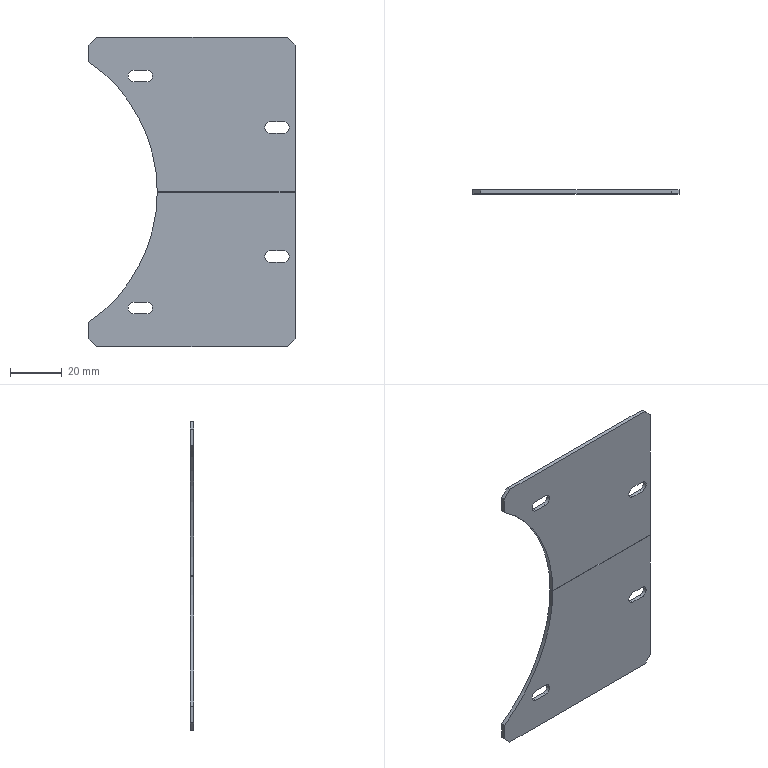Part | SolidWorks | features ICE 6, Chamfer 4, Extrusion 1 | 2 solids | 34 faces | box 80 x 1.5 x 120 mm | volume 11312 mm3 | plane 24 | cylinder 10 | commonest cylinder face diameters 4.5 x8 123 x2
STEP:
#1=CARTESIAN_POINT('',(-249.5,1.5,0.05));
#2=VERTEX_POINT('',#1);
#3=CARTESIAN_POINT('',(-196.,1.5,0.05));
#4=VERTEX_POINT('',#3);
#5=CARTESIAN_POINT('',(-276.,1.5,0.05));
#6=DIRECTION('',(1.,0.,0.));
#7=VECTOR('',#6,1000.);
#8=LINE('',#5,#7);
#9=EDGE_CURVE('',#2,#4,#8,.T.);
#10=ORIENTED_EDGE('',*,*,#9,.T.);
#11=CARTESIAN_POINT('',(-196.,0.,0.05));
#12=VERTEX_POINT('',#11);
#13=CARTESIAN_POINT('',(-196.,0.,0.05));
#14=DIRECTION('',(0.,-1.,0.));
#15=VECTOR('',#14,1000.);
#16=LINE('',#13,#15);
#17=EDGE_CURVE('',#4,#12,#16,.T.);
#18=ORIENTED_EDGE('',*,*,#17,.T.);
#19=CARTESIAN_POINT('',(-249.5,0.,0.05));
#20=VERTEX_POINT('',#19);
#21=CARTESIAN_POINT('',(-276.,0.,0.05));
#22=DIRECTION('',(1.,0.,0.));
#23=VECTOR('',#22,1000.);
#24=LINE('',#21,#23);
#25=EDGE_CURVE('',#20,#12,#24,.T.);
#26=ORIENTED_EDGE('',*,*,#25,.F.);
#27=CARTESIAN_POINT('',(-249.5,-8.5,0.05));
#28=DIRECTION('',(0.,1.,0.));
#29=VECTOR('',#28,1000.);
#30=LINE('',#27,#29);
#31=EDGE_CURVE('',#20,#2,#30,.T.);
#32=ORIENTED_EDGE('',*,*,#31,.T.);
#33=EDGE_LOOP('',(#10,#18,#26,#32));
#34=FACE_OUTER_BOUND('',#33,.T.);
#35=CARTESIAN_POINT('',(-276.,0.,0.05));
#36=DIRECTION('',(0.,0.,1.));
#37=DIRECTION('',(1.,0.,0.));
#38=AXIS2_PLACEMENT_3D('',#35,#36,#37);
#39=PLANE('',#38);
#40=ADVANCED_FACE('',(#34),#39,.F.);
#41=CARTESIAN_POINT('',(-276.,1.5,50.569));
#42=VERTEX_POINT('',#41);
#43=CARTESIAN_POINT('',(-276.,1.5,57.));
#44=VERTEX_POINT('',#43);
#45=CARTESIAN_POINT('',(-276.,1.5,-60.));
#46=DIRECTION('',(0.,0.,1.));
#47=VECTOR('',#46,1000.);
#48=LINE('',#45,#47);
#49=EDGE_CURVE('',#42,#44,#48,.T.);
#50=ORIENTED_EDGE('',*,*,#49,.F.);
#51=CARTESIAN_POINT('',(-276.,0.,50.569));
#52=VERTEX_POINT('',#51);
#53=CARTESIAN_POINT('',(-276.,-8.5,50.569));
#54=DIRECTION('',(0.,-1.,0.));
#55=VECTOR('',#54,1000.);
#56=LINE('',#53,#55);
#57=EDGE_CURVE('',#42,#52,#56,.T.);
#58=ORIENTED_EDGE('',*,*,#57,.T.);
#59=CARTESIAN_POINT('',(-276.,0.,57.));
#60=VERTEX_POINT('',#59);
#61=CARTESIAN_POINT('',(-276.,0.,-60.));
#62=DIRECTION('',(0.,0.,1.));
#63=VECTOR('',#62,1000.);
#64=LINE('',#61,#63);
#65=EDGE_CURVE('',#52,#60,#64,.T.);
#66=ORIENTED_EDGE('',*,*,#65,.T.);
#67=CARTESIAN_POINT('',(-276.,1.5,57.));
#68=DIRECTION('',(0.,1.,0.));
#69=VECTOR('',#68,1000.);
#70=LINE('',#67,#69);
#71=EDGE_CURVE('',#60,#44,#70,.T.);
#72=ORIENTED_EDGE('',*,*,#71,.T.);
#73=EDGE_LOOP('',(#50,#58,#66,#72));
#74=FACE_OUTER_BOUND('',#73,.T.);
#75=CARTESIAN_POINT('',(-276.,1.5,-60.));
#76=DIRECTION('',(1.,0.,0.));
#77=DIRECTION('',(0.,0.,-1.));
#78=AXIS2_PLACEMENT_3D('',#75,#76,#77);
#79=PLANE('',#78);
#80=ADVANCED_FACE('',(#74),#79,.F.);
#81=CARTESIAN_POINT('',(-200.5,1.5,27.25));
#82=VERTEX_POINT('',#81);
#83=CARTESIAN_POINT('',(-200.5,1.5,22.75));
#84=VERTEX_POINT('',#83);
#85=CARTESIAN_POINT('',(-200.5,1.5,25.));
#86=DIRECTION('',(0.,1.,0.));
#87=DIRECTION('',(0.,0.,1.));
#88=AXIS2_PLACEMENT_3D('',#85,#86,#87);
#89=CIRCLE('',#88,2.25);
#90=EDGE_CURVE('',#82,#84,#89,.T.);
#91=ORIENTED_EDGE('',*,*,#90,.F.);
#92=CARTESIAN_POINT('',(-205.5,1.5,27.25));
#93=VERTEX_POINT('',#92);
#94=CARTESIAN_POINT('',(0.,1.5,27.25));
#95=DIRECTION('',(1.,0.,0.));
#96=VECTOR('',#95,1000.);
#97=LINE('',#94,#96);
#98=EDGE_CURVE('',#93,#82,#97,.T.);
#99=ORIENTED_EDGE('',*,*,#98,.F.);
#100=CARTESIAN_POINT('',(-205.5,1.5,22.75));
#101=VERTEX_POINT('',#100);
#102=CARTESIAN_POINT('',(-205.5,1.5,25.));
#103=DIRECTION('',(0.,1.,0.));
#104=DIRECTION('',(0.,0.,1.));
#105=AXIS2_PLACEMENT_3D('',#102,#103,#104);
#106=CIRCLE('',#105,2.25);
#107=EDGE_CURVE('',#101,#93,#106,.T.);
#108=ORIENTED_EDGE('',*,*,#107,.F.);
#109=CARTESIAN_POINT('',(0.,1.5,22.75));
#110=DIRECTION('',(-1.,0.,0.));
#111=VECTOR('',#110,1000.);
#112=LINE('',#109,#111);
#113=EDGE_CURVE('',#84,#101,#112,.T.);
#114=ORIENTED_EDGE('',*,*,#113,.F.);
#115=EDGE_LOOP('',(#91,#99,#108,#114));
#116=FACE_BOUND('',#115,.T.);
#117=CARTESIAN_POINT('',(-273.,1.5,60.));
#118=VERTEX_POINT('',#117);
#119=CARTESIAN_POINT('',(-199.,1.5,60.));
#120=VERTEX_POINT('',#119);
#121=CARTESIAN_POINT('',(-276.,1.5,60.));
#122=DIRECTION('',(1.,0.,0.));
#123=VECTOR('',#122,1000.);
#124=LINE('',#121,#123);
#125=EDGE_CURVE('',#118,#120,#124,.T.);
#126=ORIENTED_EDGE('',*,*,#125,.T.);
#127=CARTESIAN_POINT('',(-196.,1.5,57.));
#128=VERTEX_POINT('',#127);
#129=CARTESIAN_POINT('',(-69.5,1.5,-69.5));
#130=DIRECTION('',(0.7071,0.,-0.7071));
#131=VECTOR('',#130,1000.);
#132=LINE('',#129,#131);
#133=EDGE_CURVE('',#120,#128,#132,.T.);
#134=ORIENTED_EDGE('',*,*,#133,.T.);
#135=CARTESIAN_POINT('',(-196.,1.5,0.));
#136=DIRECTION('',(0.,0.,1.));
#137=VECTOR('',#136,1000.);
#138=LINE('',#135,#137);
#139=EDGE_CURVE('',#4,#128,#138,.T.);
#140=ORIENTED_EDGE('',*,*,#139,.F.);
#141=ORIENTED_EDGE('',*,*,#9,.F.);
#142=CARTESIAN_POINT('',(-311.,1.5,0.));
#143=DIRECTION('',(0.,1.,0.));
#144=DIRECTION('',(0.,0.,1.));
#145=AXIS2_PLACEMENT_3D('',#142,#143,#144);
#146=CIRCLE('',#145,61.5);
#147=EDGE_CURVE('',#42,#2,#146,.T.);
#148=ORIENTED_EDGE('',*,*,#147,.F.);
#149=ORIENTED_EDGE('',*,*,#49,.T.);
#150=CARTESIAN_POINT('',(-166.5,1.5,166.5));
#151=DIRECTION('',(0.7071,0.,0.7071));
#152=VECTOR('',#151,1000.);
#153=LINE('',#150,#152);
#154=EDGE_CURVE('',#44,#118,#153,.T.);
#155=ORIENTED_EDGE('',*,*,#154,.T.);
#156=EDGE_LOOP('',(#126,#134,#140,#141,#148,#149,#155));
#157=FACE_OUTER_BOUND('',#156,.T.);
#158=CARTESIAN_POINT('',(-258.5,1.5,42.75));
#159=VERTEX_POINT('',#158);
#160=CARTESIAN_POINT('',(-258.5,1.5,47.25));
#161=VERTEX_POINT('',#160);
#162=CARTESIAN_POINT('',(-258.5,1.5,45.));
#163=DIRECTION('',(0.,1.,0.));
#164=DIRECTION('',(0.,0.,1.));
#165=AXIS2_PLACEMENT_3D('',#162,#163,#164);
#166=CIRCLE('',#165,2.25);
#167=EDGE_CURVE('',#159,#161,#166,.T.);
#168=ORIENTED_EDGE('',*,*,#167,.F.);
#169=CARTESIAN_POINT('',(-253.5,1.5,42.75));
#170=VERTEX_POINT('',#169);
#171=CARTESIAN_POINT('',(-258.5,1.5,42.75));
#172=DIRECTION('',(-1.,0.,0.));
#173=VECTOR('',#172,1000.);
#174=LINE('',#171,#173);
#175=EDGE_CURVE('',#170,#159,#174,.T.);
#176=ORIENTED_EDGE('',*,*,#175,.F.);
#177=CARTESIAN_POINT('',(-253.5,1.5,47.25));
#178=VERTEX_POINT('',#177);
#179=CARTESIAN_POINT('',(-253.5,1.5,45.));
#180=DIRECTION('',(0.,1.,0.));
#181=DIRECTION('',(0.,0.,1.));
#182=AXIS2_PLACEMENT_3D('',#179,#180,#181);
#183=CIRCLE('',#182,2.25);
#184=EDGE_CURVE('',#178,#170,#183,.T.);
#185=ORIENTED_EDGE('',*,*,#184,.F.);
#186=CARTESIAN_POINT('',(-258.5,1.5,47.25));
#187=DIRECTION('',(1.,0.,0.));
#188=VECTOR('',#187,1000.);
#189=LINE('',#186,#188);
#190=EDGE_CURVE('',#161,#178,#189,.T.);
#191=ORIENTED_EDGE('',*,*,#190,.F.);
#192=EDGE_LOOP('',(#168,#176,#185,#191));
#193=FACE_BOUND('',#192,.T.);
#194=CARTESIAN_POINT('',(0.,1.5,0.));
#195=DIRECTION('',(0.,1.,0.));
#196=DIRECTION('',(0.,0.,1.));
#197=AXIS2_PLACEMENT_3D('',#194,#195,#196);
#198=PLANE('',#197);
#199=ADVANCED_FACE('',(#116,#157,#193),#198,.T.);
#200=CARTESIAN_POINT('',(-200.5,0.,27.25));
#201=VERTEX_POINT('',#200);
#202=CARTESIAN_POINT('',(-205.5,0.,27.25));
#203=VERTEX_POINT('',#202);
#204=CARTESIAN_POINT('',(-200.5,0.,27.25));
#205=DIRECTION('',(-1.,0.,0.));
#206=VECTOR('',#205,1000.);
#207=LINE('',#204,#206);
#208=EDGE_CURVE('',#201,#203,#207,.T.);
#209=ORIENTED_EDGE('',*,*,#208,.F.);
#210=CARTESIAN_POINT('',(-200.5,0.,22.75));
#211=VERTEX_POINT('',#210);
#212=CARTESIAN_POINT('',(-200.5,0.,25.));
#213=DIRECTION('',(0.,-1.,0.));
#214=DIRECTION('',(0.,0.,-1.));
#215=AXIS2_PLACEMENT_3D('',#212,#213,#214);
#216=CIRCLE('',#215,2.25);
#217=EDGE_CURVE('',#211,#201,#216,.T.);
#218=ORIENTED_EDGE('',*,*,#217,.F.);
#219=CARTESIAN_POINT('',(-205.5,0.,22.75));
#220=VERTEX_POINT('',#219);
#221=CARTESIAN_POINT('',(-200.5,0.,22.75));
#222=DIRECTION('',(1.,0.,0.));
#223=VECTOR('',#222,1000.);
#224=LINE('',#221,#223);
#225=EDGE_CURVE('',#220,#211,#224,.T.);
#226=ORIENTED_EDGE('',*,*,#225,.F.);
#227=CARTESIAN_POINT('',(-205.5,0.,25.));
#228=DIRECTION('',(0.,-1.,0.));
#229=DIRECTION('',(0.,0.,-1.));
#230=AXIS2_PLACEMENT_3D('',#227,#228,#229);
#231=CIRCLE('',#230,2.25);
#232=EDGE_CURVE('',#203,#220,#231,.T.);
#233=ORIENTED_EDGE('',*,*,#232,.F.);
#234=EDGE_LOOP('',(#209,#218,#226,#233));
#235=FACE_BOUND('',#234,.T.);
#236=CARTESIAN_POINT('',(-196.,0.,57.));
#237=VERTEX_POINT('',#236);
#238=CARTESIAN_POINT('',(-196.,0.,126.432));
#239=DIRECTION('',(0.,0.,-1.));
#240=VECTOR('',#239,1000.);
#241=LINE('',#238,#240);
#242=EDGE_CURVE('',#237,#12,#241,.T.);
#243=ORIENTED_EDGE('',*,*,#242,.F.);
#244=CARTESIAN_POINT('',(-199.,0.,60.));
#245=VERTEX_POINT('',#244);
#246=CARTESIAN_POINT('',(-199.,0.,60.));
#247=DIRECTION('',(-0.7071,0.,0.7071));
#248=VECTOR('',#247,1000.);
#249=LINE('',#246,#248);
#250=EDGE_CURVE('',#237,#245,#249,.T.);
#251=ORIENTED_EDGE('',*,*,#250,.T.);
#252=CARTESIAN_POINT('',(-273.,0.,60.));
#253=VERTEX_POINT('',#252);
#254=CARTESIAN_POINT('',(-276.,0.,60.));
#255=DIRECTION('',(1.,0.,0.));
#256=VECTOR('',#255,1000.);
#257=LINE('',#254,#256);
#258=EDGE_CURVE('',#253,#245,#257,.T.);
#259=ORIENTED_EDGE('',*,*,#258,.F.);
#260=CARTESIAN_POINT('',(-273.,0.,60.));
#261=DIRECTION('',(-0.7071,0.,-0.7071));
#262=VECTOR('',#261,1000.);
#263=LINE('',#260,#262);
#264=EDGE_CURVE('',#253,#60,#263,.T.);
#265=ORIENTED_EDGE('',*,*,#264,.T.);
#266=ORIENTED_EDGE('',*,*,#65,.F.);
#267=CARTESIAN_POINT('',(-311.,0.,0.));
#268=DIRECTION('',(0.,1.,0.));
#269=DIRECTION('',(0.,0.,1.));
#270=AXIS2_PLACEMENT_3D('',#267,#268,#269);
#271=CIRCLE('',#270,61.5);
#272=EDGE_CURVE('',#52,#20,#271,.T.);
#273=ORIENTED_EDGE('',*,*,#272,.T.);
#274=ORIENTED_EDGE('',*,*,#25,.T.);
#275=EDGE_LOOP('',(#243,#251,#259,#265,#266,#273,#274));
#276=FACE_OUTER_BOUND('',#275,.T.);
#277=CARTESIAN_POINT('',(-253.5,0.,42.75));
#278=VERTEX_POINT('',#277);
#279=CARTESIAN_POINT('',(-258.5,0.,42.75));
#280=VERTEX_POINT('',#279);
#281=CARTESIAN_POINT('',(-258.5,0.,42.75));
#282=DIRECTION('',(-1.,0.,0.));
#283=VECTOR('',#282,1000.);
#284=LINE('',#281,#283);
#285=EDGE_CURVE('',#278,#280,#284,.T.);
#286=ORIENTED_EDGE('',*,*,#285,.T.);
#287=CARTESIAN_POINT('',(-258.5,0.,47.25));
#288=VERTEX_POINT('',#287);
#289=CARTESIAN_POINT('',(-258.5,0.,45.));
#290=DIRECTION('',(0.,1.,0.));
#291=DIRECTION('',(0.,0.,1.));
#292=AXIS2_PLACEMENT_3D('',#289,#290,#291);
#293=CIRCLE('',#292,2.25);
#294=EDGE_CURVE('',#280,#288,#293,.T.);
#295=ORIENTED_EDGE('',*,*,#294,.T.);
#296=CARTESIAN_POINT('',(-253.5,0.,47.25));
#297=VERTEX_POINT('',#296);
#298=CARTESIAN_POINT('',(-258.5,0.,47.25));
#299=DIRECTION('',(1.,0.,0.));
#300=VECTOR('',#299,1000.);
#301=LINE('',#298,#300);
#302=EDGE_CURVE('',#288,#297,#301,.T.);
#303=ORIENTED_EDGE('',*,*,#302,.T.);
#304=CARTESIAN_POINT('',(-253.5,0.,45.));
#305=DIRECTION('',(0.,1.,0.));
#306=DIRECTION('',(0.,0.,1.));
#307=AXIS2_PLACEMENT_3D('',#304,#305,#306);
#308=CIRCLE('',#307,2.25);
#309=EDGE_CURVE('',#297,#278,#308,.T.);
#310=ORIENTED_EDGE('',*,*,#309,.T.);
#311=EDGE_LOOP('',(#286,#295,#303,#310));
#312=FACE_BOUND('',#311,.T.);
#313=CARTESIAN_POINT('',(0.,0.,0.));
#314=DIRECTION('',(0.,1.,0.));
#315=DIRECTION('',(0.,0.,1.));
#316=AXIS2_PLACEMENT_3D('',#313,#314,#315);
#317=PLANE('',#316);
#318=ADVANCED_FACE('',(#235,#276,#312),#317,.F.);
#319=ORIENTED_EDGE('',*,*,#258,.T.);
#320=CARTESIAN_POINT('',(-199.,1.5,60.));
#321=DIRECTION('',(0.,1.,0.));
#322=VECTOR('',#321,1000.);
#323=LINE('',#320,#322);
#324=EDGE_CURVE('',#245,#120,#323,.T.);
#325=ORIENTED_EDGE('',*,*,#324,.T.);
#326=ORIENTED_EDGE('',*,*,#125,.F.);
#327=CARTESIAN_POINT('',(-273.,1.5,60.));
#328=DIRECTION('',(0.,-1.,0.));
#329=VECTOR('',#328,1000.);
#330=LINE('',#327,#329);
#331=EDGE_CURVE('',#118,#253,#330,.T.);
#332=ORIENTED_EDGE('',*,*,#331,.T.);
#333=EDGE_LOOP('',(#319,#325,#326,#332));
#334=FACE_OUTER_BOUND('',#333,.T.);
#335=CARTESIAN_POINT('',(-276.,1.5,60.));
#336=DIRECTION('',(0.,0.,-1.));
#337=DIRECTION('',(-1.,0.,0.));
#338=AXIS2_PLACEMENT_3D('',#335,#336,#337);
#339=PLANE('',#338);
#340=ADVANCED_FACE('',(#334),#339,.F.);
#341=ORIENTED_EDGE('',*,*,#154,.F.);
#342=ORIENTED_EDGE('',*,*,#71,.F.);
#343=ORIENTED_EDGE('',*,*,#264,.F.);
#344=ORIENTED_EDGE('',*,*,#331,.F.);
#345=EDGE_LOOP('',(#341,#342,#343,#344));
#346=FACE_OUTER_BOUND('',#345,.T.);
#347=CARTESIAN_POINT('',(-273.,1.5,60.));
#348=DIRECTION('',(0.7071,0.,-0.7071));
#349=DIRECTION('',(0.,-1.,0.));
#350=AXIS2_PLACEMENT_3D('',#347,#348,#349);
#351=PLANE('',#350);
#352=ADVANCED_FACE('',(#346),#351,.F.);
#353=ORIENTED_EDGE('',*,*,#167,.T.);
#354=CARTESIAN_POINT('',(-258.5,0.,47.25));
#355=DIRECTION('',(0.,1.,0.));
#356=VECTOR('',#355,1000.);
#357=LINE('',#354,#356);
#358=EDGE_CURVE('',#288,#161,#357,.T.);
#359=ORIENTED_EDGE('',*,*,#358,.F.);
#360=ORIENTED_EDGE('',*,*,#294,.F.);
#361=CARTESIAN_POINT('',(-258.5,0.,42.75));
#362=DIRECTION('',(0.,1.,0.));
#363=VECTOR('',#362,1000.);
#364=LINE('',#361,#363);
#365=EDGE_CURVE('',#280,#159,#364,.T.);
#366=ORIENTED_EDGE('',*,*,#365,.T.);
#367=EDGE_LOOP('',(#353,#359,#360,#366));
#368=FACE_OUTER_BOUND('',#367,.T.);
#369=CARTESIAN_POINT('',(-258.5,0.,45.));
#370=DIRECTION('',(0.,1.,0.));
#371=DIRECTION('',(0.,0.,1.));
#372=AXIS2_PLACEMENT_3D('',#369,#370,#371);
#373=CYLINDRICAL_SURFACE('',#372,2.25);
#374=ADVANCED_FACE('',(#368),#373,.F.);
#375=ORIENTED_EDGE('',*,*,#175,.T.);
#376=ORIENTED_EDGE('',*,*,#365,.F.);
#377=ORIENTED_EDGE('',*,*,#285,.F.);
#378=CARTESIAN_POINT('',(-253.5,0.,42.75));
#379=DIRECTION('',(0.,1.,0.));
#380=VECTOR('',#379,1000.);
#381=LINE('',#378,#380);
#382=EDGE_CURVE('',#278,#170,#381,.T.);
#383=ORIENTED_EDGE('',*,*,#382,.T.);
#384=EDGE_LOOP('',(#375,#376,#377,#383));
#385=FACE_OUTER_BOUND('',#384,.T.);
#386=CARTESIAN_POINT('',(-258.5,0.,42.75));
#387=DIRECTION('',(0.,0.,-1.));
#388=DIRECTION('',(-1.,0.,0.));
#389=AXIS2_PLACEMENT_3D('',#386,#387,#388);
#390=PLANE('',#389);
#391=ADVANCED_FACE('',(#385),#390,.F.);
#392=ORIENTED_EDGE('',*,*,#184,.T.);
#393=ORIENTED_EDGE('',*,*,#382,.F.);
#394=ORIENTED_EDGE('',*,*,#309,.F.);
#395=CARTESIAN_POINT('',(-253.5,0.,47.25));
#396=DIRECTION('',(0.,1.,0.));
#397=VECTOR('',#396,1000.);
#398=LINE('',#395,#397);
#399=EDGE_CURVE('',#297,#178,#398,.T.);
#400=ORIENTED_EDGE('',*,*,#399,.T.);
#401=EDGE_LOOP('',(#392,#393,#394,#400));
#402=FACE_OUTER_BOUND('',#401,.T.);
#403=CARTESIAN_POINT('',(-253.5,0.,45.));
#404=DIRECTION('',(0.,1.,0.));
#405=DIRECTION('',(0.,0.,1.));
#406=AXIS2_PLACEMENT_3D('',#403,#404,#405);
#407=CYLINDRICAL_SURFACE('',#406,2.25);
#408=ADVANCED_FACE('',(#402),#407,.F.);
#409=ORIENTED_EDGE('',*,*,#190,.T.);
#410=ORIENTED_EDGE('',*,*,#399,.F.);
#411=ORIENTED_EDGE('',*,*,#302,.F.);
#412=ORIENTED_EDGE('',*,*,#358,.T.);
#413=EDGE_LOOP('',(#409,#410,#411,#412));
#414=FACE_OUTER_BOUND('',#413,.T.);
#415=CARTESIAN_POINT('',(-258.5,0.,47.25));
#416=DIRECTION('',(0.,0.,1.));
#417=DIRECTION('',(1.,0.,0.));
#418=AXIS2_PLACEMENT_3D('',#415,#416,#417);
#419=PLANE('',#418);
#420=ADVANCED_FACE('',(#414),#419,.F.);
#421=ORIENTED_EDGE('',*,*,#272,.F.);
#422=ORIENTED_EDGE('',*,*,#57,.F.);
#423=ORIENTED_EDGE('',*,*,#147,.T.);
#424=ORIENTED_EDGE('',*,*,#31,.F.);
#425=EDGE_LOOP('',(#421,#422,#423,#424));
#426=FACE_OUTER_BOUND('',#425,.T.);
#427=CARTESIAN_POINT('',(-311.,-8.5,0.));
#428=DIRECTION('',(0.,1.,0.));
#429=DIRECTION('',(0.,0.,1.));
#430=AXIS2_PLACEMENT_3D('',#427,#428,#429);
#431=CYLINDRICAL_SURFACE('',#430,61.5);
#432=ADVANCED_FACE('',(#426),#431,.F.);
#433=ORIENTED_EDGE('',*,*,#139,.T.);
#434=CARTESIAN_POINT('',(-196.,10.,57.));
#435=DIRECTION('',(0.,-1.,0.));
#436=VECTOR('',#435,1000.);
#437=LINE('',#434,#436);
#438=EDGE_CURVE('',#128,#237,#437,.T.);
#439=ORIENTED_EDGE('',*,*,#438,.T.);
#440=ORIENTED_EDGE('',*,*,#242,.T.);
#441=ORIENTED_EDGE('',*,*,#17,.F.);
#442=EDGE_LOOP('',(#433,#439,#440,#441));
#443=FACE_OUTER_BOUND('',#442,.T.);
#444=CARTESIAN_POINT('',(-196.,10.,126.432));
#445=DIRECTION('',(-1.,0.,0.));
#446=DIRECTION('',(0.,0.,1.));
#447=AXIS2_PLACEMENT_3D('',#444,#445,#446);
#448=PLANE('',#447);
#449=ADVANCED_FACE('',(#443),#448,.F.);
#450=ORIENTED_EDGE('',*,*,#90,.T.);
#451=CARTESIAN_POINT('',(-200.5,10.,22.75));
#452=DIRECTION('',(0.,-1.,0.));
#453=VECTOR('',#452,1000.);
#454=LINE('',#451,#453);
#455=EDGE_CURVE('',#84,#211,#454,.T.);
#456=ORIENTED_EDGE('',*,*,#455,.T.);
#457=ORIENTED_EDGE('',*,*,#217,.T.);
#458=CARTESIAN_POINT('',(-200.5,10.,27.25));
#459=DIRECTION('',(0.,-1.,0.));
#460=VECTOR('',#459,1000.);
#461=LINE('',#458,#460);
#462=EDGE_CURVE('',#82,#201,#461,.T.);
#463=ORIENTED_EDGE('',*,*,#462,.F.);
#464=EDGE_LOOP('',(#450,#456,#457,#463));
#465=FACE_OUTER_BOUND('',#464,.T.);
#466=CARTESIAN_POINT('',(-200.5,10.,25.));
#467=DIRECTION('',(0.,-1.,0.));
#468=DIRECTION('',(0.,0.,-1.));
#469=AXIS2_PLACEMENT_3D('',#466,#467,#468);
#470=CYLINDRICAL_SURFACE('',#469,2.25);
#471=ADVANCED_FACE('',(#465),#470,.F.);
#472=ORIENTED_EDGE('',*,*,#113,.T.);
#473=CARTESIAN_POINT('',(-205.5,10.,22.75));
#474=DIRECTION('',(0.,-1.,0.));
#475=VECTOR('',#474,1000.);
#476=LINE('',#473,#475);
#477=EDGE_CURVE('',#101,#220,#476,.T.);
#478=ORIENTED_EDGE('',*,*,#477,.T.);
#479=ORIENTED_EDGE('',*,*,#225,.T.);
#480=ORIENTED_EDGE('',*,*,#455,.F.);
#481=EDGE_LOOP('',(#472,#478,#479,#480));
#482=FACE_OUTER_BOUND('',#481,.T.);
#483=CARTESIAN_POINT('',(-200.5,10.,22.75));
#484=DIRECTION('',(0.,0.,-1.));
#485=DIRECTION('',(-1.,0.,0.));
#486=AXIS2_PLACEMENT_3D('',#483,#484,#485);
#487=PLANE('',#486);
#488=ADVANCED_FACE('',(#482),#487,.F.);
#489=ORIENTED_EDGE('',*,*,#107,.T.);
#490=CARTESIAN_POINT('',(-205.5,10.,27.25));
#491=DIRECTION('',(0.,-1.,0.));
#492=VECTOR('',#491,1000.);
#493=LINE('',#490,#492);
#494=EDGE_CURVE('',#93,#203,#493,.T.);
#495=ORIENTED_EDGE('',*,*,#494,.T.);
#496=ORIENTED_EDGE('',*,*,#232,.T.);
#497=ORIENTED_EDGE('',*,*,#477,.F.);
#498=EDGE_LOOP('',(#489,#495,#496,#497));
#499=FACE_OUTER_BOUND('',#498,.T.);
#500=CARTESIAN_POINT('',(-205.5,10.,25.));
#501=DIRECTION('',(0.,-1.,0.));
#502=DIRECTION('',(0.,0.,-1.));
#503=AXIS2_PLACEMENT_3D('',#500,#501,#502);
#504=CYLINDRICAL_SURFACE('',#503,2.25);
#505=ADVANCED_FACE('',(#499),#504,.F.);
#506=ORIENTED_EDGE('',*,*,#98,.T.);
#507=ORIENTED_EDGE('',*,*,#462,.T.);
#508=ORIENTED_EDGE('',*,*,#208,.T.);
#509=ORIENTED_EDGE('',*,*,#494,.F.);
#510=EDGE_LOOP('',(#506,#507,#508,#509));
#511=FACE_OUTER_BOUND('',#510,.T.);
#512=CARTESIAN_POINT('',(-200.5,10.,27.25));
#513=DIRECTION('',(0.,0.,1.));
#514=DIRECTION('',(1.,0.,0.));
#515=AXIS2_PLACEMENT_3D('',#512,#513,#514);
#516=PLANE('',#515);
#517=ADVANCED_FACE('',(#511),#516,.F.);
#518=ORIENTED_EDGE('',*,*,#250,.F.);
#519=ORIENTED_EDGE('',*,*,#438,.F.);
#520=ORIENTED_EDGE('',*,*,#133,.F.);
#521=ORIENTED_EDGE('',*,*,#324,.F.);
#522=EDGE_LOOP('',(#518,#519,#520,#521));
#523=FACE_OUTER_BOUND('',#522,.T.);
#524=CARTESIAN_POINT('',(-199.,1.5,60.));
#525=DIRECTION('',(-0.7071,0.,-0.7071));
#526=DIRECTION('',(0.,1.,0.));
#527=AXIS2_PLACEMENT_3D('',#524,#525,#526);
#528=PLANE('',#527);
#529=ADVANCED_FACE('',(#523),#528,.F.);
#530=CLOSED_SHELL('',(#40,#80,#199,#318,#340,#352,#374,#391,#408,#420,#432,#449,#471,#488,#505,#517,#529));
#531=MANIFOLD_SOLID_BREP('',#530);
#532=CARTESIAN_POINT('',(-196.,0.,-0.05));
#533=VERTEX_POINT('',#532);
#534=CARTESIAN_POINT('',(-249.5,0.,-0.05));
#535=VERTEX_POINT('',#534);
#536=CARTESIAN_POINT('',(-276.,0.,-0.05));
#537=DIRECTION('',(-1.,0.,0.));
#538=VECTOR('',#537,1000.);
#539=LINE('',#536,#538);
#540=EDGE_CURVE('',#533,#535,#539,.T.);
#541=ORIENTED_EDGE('',*,*,#540,.F.);
#542=CARTESIAN_POINT('',(-196.,1.5,-0.05));
#543=VERTEX_POINT('',#542);
#544=CARTESIAN_POINT('',(-196.,0.,-0.05));
#545=DIRECTION('',(0.,1.,0.));
#546=VECTOR('',#545,1000.);
#547=LINE('',#544,#546);
#548=EDGE_CURVE('',#533,#543,#547,.T.);
#549=ORIENTED_EDGE('',*,*,#548,.T.);
#550=CARTESIAN_POINT('',(-249.5,1.5,-0.05));
#551=VERTEX_POINT('',#550);
#552=CARTESIAN_POINT('',(-276.,1.5,-0.05));
#553=DIRECTION('',(-1.,0.,0.));
#554=VECTOR('',#553,1000.);
#555=LINE('',#552,#554);
#556=EDGE_CURVE('',#543,#551,#555,.T.);
#557=ORIENTED_EDGE('',*,*,#556,.T.);
#558=CARTESIAN_POINT('',(-249.5,-8.5,-0.05));
#559=DIRECTION('',(0.,-1.,0.));
#560=VECTOR('',#559,1000.);
#561=LINE('',#558,#560);
#562=EDGE_CURVE('',#551,#535,#561,.T.);
#563=ORIENTED_EDGE('',*,*,#562,.T.);
#564=EDGE_LOOP('',(#541,#549,#557,#563));
#565=FACE_OUTER_BOUND('',#564,.T.);
#566=CARTESIAN_POINT('',(-276.,0.,-0.05));
#567=DIRECTION('',(0.,0.,-1.));
#568=DIRECTION('',(-1.,0.,0.));
#569=AXIS2_PLACEMENT_3D('',#566,#567,#568);
#570=PLANE('',#569);
#571=ADVANCED_FACE('',(#565),#570,.F.);
#572=CARTESIAN_POINT('',(-199.,1.5,-60.));
#573=VERTEX_POINT('',#572);
#574=CARTESIAN_POINT('',(-273.,1.5,-60.));
#575=VERTEX_POINT('',#574);
#576=CARTESIAN_POINT('',(-276.,1.5,-60.));
#577=DIRECTION('',(-1.,0.,0.));
#578=VECTOR('',#577,1000.);
#579=LINE('',#576,#578);
#580=EDGE_CURVE('',#573,#575,#579,.T.);
#581=ORIENTED_EDGE('',*,*,#580,.F.);
#582=CARTESIAN_POINT('',(-199.,0.,-60.));
#583=VERTEX_POINT('',#582);
#584=CARTESIAN_POINT('',(-199.,1.5,-60.));
#585=DIRECTION('',(0.,-1.,0.));
#586=VECTOR('',#585,1000.);
#587=LINE('',#584,#586);
#588=EDGE_CURVE('',#573,#583,#587,.T.);
#589=ORIENTED_EDGE('',*,*,#588,.T.);
#590=CARTESIAN_POINT('',(-273.,0.,-60.));
#591=VERTEX_POINT('',#590);
#592=CARTESIAN_POINT('',(-276.,0.,-60.));
#593=DIRECTION('',(-1.,0.,0.));
#594=VECTOR('',#593,1000.);
#595=LINE('',#592,#594);
#596=EDGE_CURVE('',#583,#591,#595,.T.);
#597=ORIENTED_EDGE('',*,*,#596,.T.);
#598=CARTESIAN_POINT('',(-273.,1.5,-60.));
#599=DIRECTION('',(0.,1.,0.));
#600=VECTOR('',#599,1000.);
#601=LINE('',#598,#600);
#602=EDGE_CURVE('',#591,#575,#601,.T.);
#603=ORIENTED_EDGE('',*,*,#602,.T.);
#604=EDGE_LOOP('',(#581,#589,#597,#603));
#605=FACE_OUTER_BOUND('',#604,.T.);
#606=CARTESIAN_POINT('',(-276.,1.5,-60.));
#607=DIRECTION('',(0.,0.,1.));
#608=DIRECTION('',(1.,0.,0.));
#609=AXIS2_PLACEMENT_3D('',#606,#607,#608);
#610=PLANE('',#609);
#611=ADVANCED_FACE('',(#605),#610,.F.);
#612=CARTESIAN_POINT('',(-276.,1.5,-57.));
#613=VERTEX_POINT('',#612);
#614=CARTESIAN_POINT('',(-166.5,1.5,-166.5));
#615=DIRECTION('',(-0.7071,0.,0.7071));
#616=VECTOR('',#615,1000.);
#617=LINE('',#614,#616);
#618=EDGE_CURVE('',#575,#613,#617,.T.);
#619=ORIENTED_EDGE('',*,*,#618,.F.);
#620=ORIENTED_EDGE('',*,*,#602,.F.);
#621=CARTESIAN_POINT('',(-276.,0.,-57.));
#622=VERTEX_POINT('',#621);
#623=CARTESIAN_POINT('',(-276.,0.,-57.));
#624=DIRECTION('',(0.7071,0.,-0.7071));
#625=VECTOR('',#624,1000.);
#626=LINE('',#623,#625);
#627=EDGE_CURVE('',#622,#591,#626,.T.);
#628=ORIENTED_EDGE('',*,*,#627,.F.);
#629=CARTESIAN_POINT('',(-276.,1.5,-57.));
#630=DIRECTION('',(0.,-1.,0.));
#631=VECTOR('',#630,1000.);
#632=LINE('',#629,#631);
#633=EDGE_CURVE('',#613,#622,#632,.T.);
#634=ORIENTED_EDGE('',*,*,#633,.F.);
#635=EDGE_LOOP('',(#619,#620,#628,#634));
#636=FACE_OUTER_BOUND('',#635,.T.);
#637=CARTESIAN_POINT('',(-276.,1.5,-57.));
#638=DIRECTION('',(0.7071,0.,0.7071));
#639=DIRECTION('',(0.,-1.,0.));
#640=AXIS2_PLACEMENT_3D('',#637,#638,#639);
#641=PLANE('',#640);
#642=ADVANCED_FACE('',(#636),#641,.F.);
#643=CARTESIAN_POINT('',(-253.5,1.5,-42.75));
#644=VERTEX_POINT('',#643);
#645=CARTESIAN_POINT('',(-253.5,1.5,-47.25));
#646=VERTEX_POINT('',#645);
#647=CARTESIAN_POINT('',(-253.5,1.5,-45.));
#648=DIRECTION('',(0.,1.,0.));
#649=DIRECTION('',(0.,0.,1.));
#650=AXIS2_PLACEMENT_3D('',#647,#648,#649);
#651=CIRCLE('',#650,2.25);
#652=EDGE_CURVE('',#644,#646,#651,.T.);
#653=ORIENTED_EDGE('',*,*,#652,.T.);
#654=CARTESIAN_POINT('',(-253.5,0.,-47.25));
#655=VERTEX_POINT('',#654);
#656=CARTESIAN_POINT('',(-253.5,0.,-47.25));
#657=DIRECTION('',(0.,1.,0.));
#658=VECTOR('',#657,1000.);
#659=LINE('',#656,#658);
#660=EDGE_CURVE('',#655,#646,#659,.T.);
#661=ORIENTED_EDGE('',*,*,#660,.F.);
#662=CARTESIAN_POINT('',(-253.5,0.,-42.75));
#663=VERTEX_POINT('',#662);
#664=CARTESIAN_POINT('',(-253.5,0.,-45.));
#665=DIRECTION('',(0.,1.,0.));
#666=DIRECTION('',(0.,0.,1.));
#667=AXIS2_PLACEMENT_3D('',#664,#665,#666);
#668=CIRCLE('',#667,2.25);
#669=EDGE_CURVE('',#663,#655,#668,.T.);
#670=ORIENTED_EDGE('',*,*,#669,.F.);
#671=CARTESIAN_POINT('',(-253.5,0.,-42.75));
#672=DIRECTION('',(0.,1.,0.));
#673=VECTOR('',#672,1000.);
#674=LINE('',#671,#673);
#675=EDGE_CURVE('',#663,#644,#674,.T.);
#676=ORIENTED_EDGE('',*,*,#675,.T.);
#677=EDGE_LOOP('',(#653,#661,#670,#676));
#678=FACE_OUTER_BOUND('',#677,.T.);
#679=CARTESIAN_POINT('',(-253.5,0.,-45.));
#680=DIRECTION('',(0.,1.,0.));
#681=DIRECTION('',(0.,0.,1.));
#682=AXIS2_PLACEMENT_3D('',#679,#680,#681);
#683=CYLINDRICAL_SURFACE('',#682,2.25);
#684=ADVANCED_FACE('',(#678),#683,.F.);
#685=CARTESIAN_POINT('',(-258.5,1.5,-42.75));
#686=VERTEX_POINT('',#685);
#687=CARTESIAN_POINT('',(-258.5,1.5,-42.75));
#688=DIRECTION('',(1.,0.,0.));
#689=VECTOR('',#688,1000.);
#690=LINE('',#687,#689);
#691=EDGE_CURVE('',#686,#644,#690,.T.);
#692=ORIENTED_EDGE('',*,*,#691,.T.);
#693=ORIENTED_EDGE('',*,*,#675,.F.);
#694=CARTESIAN_POINT('',(-258.5,0.,-42.75));
#695=VERTEX_POINT('',#694);
#696=CARTESIAN_POINT('',(-258.5,0.,-42.75));
#697=DIRECTION('',(1.,0.,0.));
#698=VECTOR('',#697,1000.);
#699=LINE('',#696,#698);
#700=EDGE_CURVE('',#695,#663,#699,.T.);
#701=ORIENTED_EDGE('',*,*,#700,.F.);
#702=CARTESIAN_POINT('',(-258.5,0.,-42.75));
#703=DIRECTION('',(0.,1.,0.));
#704=VECTOR('',#703,1000.);
#705=LINE('',#702,#704);
#706=EDGE_CURVE('',#695,#686,#705,.T.);
#707=ORIENTED_EDGE('',*,*,#706,.T.);
#708=EDGE_LOOP('',(#692,#693,#701,#707));
#709=FACE_OUTER_BOUND('',#708,.T.);
#710=CARTESIAN_POINT('',(-258.5,0.,-42.75));
#711=DIRECTION('',(0.,0.,1.));
#712=DIRECTION('',(1.,0.,0.));
#713=AXIS2_PLACEMENT_3D('',#710,#711,#712);
#714=PLANE('',#713);
#715=ADVANCED_FACE('',(#709),#714,.F.);
#716=CARTESIAN_POINT('',(-258.5,1.5,-47.25));
#717=VERTEX_POINT('',#716);
#718=CARTESIAN_POINT('',(-258.5,1.5,-45.));
#719=DIRECTION('',(0.,1.,0.));
#720=DIRECTION('',(0.,0.,1.));
#721=AXIS2_PLACEMENT_3D('',#718,#719,#720);
#722=CIRCLE('',#721,2.25);
#723=EDGE_CURVE('',#717,#686,#722,.T.);
#724=ORIENTED_EDGE('',*,*,#723,.T.);
#725=ORIENTED_EDGE('',*,*,#706,.F.);
#726=CARTESIAN_POINT('',(-258.5,0.,-47.25));
#727=VERTEX_POINT('',#726);
#728=CARTESIAN_POINT('',(-258.5,0.,-45.));
#729=DIRECTION('',(0.,1.,0.));
#730=DIRECTION('',(0.,0.,1.));
#731=AXIS2_PLACEMENT_3D('',#728,#729,#730);
#732=CIRCLE('',#731,2.25);
#733=EDGE_CURVE('',#727,#695,#732,.T.);
#734=ORIENTED_EDGE('',*,*,#733,.F.);
#735=CARTESIAN_POINT('',(-258.5,0.,-47.25));
#736=DIRECTION('',(0.,1.,0.));
#737=VECTOR('',#736,1000.);
#738=LINE('',#735,#737);
#739=EDGE_CURVE('',#727,#717,#738,.T.);
#740=ORIENTED_EDGE('',*,*,#739,.T.);
#741=EDGE_LOOP('',(#724,#725,#734,#740));
#742=FACE_OUTER_BOUND('',#741,.T.);
#743=CARTESIAN_POINT('',(-258.5,0.,-45.));
#744=DIRECTION('',(0.,1.,0.));
#745=DIRECTION('',(0.,0.,1.));
#746=AXIS2_PLACEMENT_3D('',#743,#744,#745);
#747=CYLINDRICAL_SURFACE('',#746,2.25);
#748=ADVANCED_FACE('',(#742),#747,.F.);
#749=CARTESIAN_POINT('',(-258.5,1.5,-47.25));
#750=DIRECTION('',(-1.,0.,0.));
#751=VECTOR('',#750,1000.);
#752=LINE('',#749,#751);
#753=EDGE_CURVE('',#646,#717,#752,.T.);
#754=ORIENTED_EDGE('',*,*,#753,.T.);
#755=ORIENTED_EDGE('',*,*,#739,.F.);
#756=CARTESIAN_POINT('',(-258.5,0.,-47.25));
#757=DIRECTION('',(-1.,0.,0.));
#758=VECTOR('',#757,1000.);
#759=LINE('',#756,#758);
#760=EDGE_CURVE('',#655,#727,#759,.T.);
#761=ORIENTED_EDGE('',*,*,#760,.F.);
#762=ORIENTED_EDGE('',*,*,#660,.T.);
#763=EDGE_LOOP('',(#754,#755,#761,#762));
#764=FACE_OUTER_BOUND('',#763,.T.);
#765=CARTESIAN_POINT('',(-258.5,0.,-47.25));
#766=DIRECTION('',(0.,0.,-1.));
#767=DIRECTION('',(-1.,0.,0.));
#768=AXIS2_PLACEMENT_3D('',#765,#766,#767);
#769=PLANE('',#768);
#770=ADVANCED_FACE('',(#764),#769,.F.);
#771=CARTESIAN_POINT('',(-200.5,1.5,-22.75));
#772=VERTEX_POINT('',#771);
#773=CARTESIAN_POINT('',(-200.5,1.5,-27.25));
#774=VERTEX_POINT('',#773);
#775=CARTESIAN_POINT('',(-200.5,1.5,-25.));
#776=DIRECTION('',(0.,1.,0.));
#777=DIRECTION('',(0.,0.,1.));
#778=AXIS2_PLACEMENT_3D('',#775,#776,#777);
#779=CIRCLE('',#778,2.25);
#780=EDGE_CURVE('',#772,#774,#779,.T.);
#781=ORIENTED_EDGE('',*,*,#780,.F.);
#782=CARTESIAN_POINT('',(-205.5,1.5,-22.75));
#783=VERTEX_POINT('',#782);
#784=CARTESIAN_POINT('',(0.,1.5,-22.75));
#785=DIRECTION('',(1.,0.,0.));
#786=VECTOR('',#785,1000.);
#787=LINE('',#784,#786);
#788=EDGE_CURVE('',#783,#772,#787,.T.);
#789=ORIENTED_EDGE('',*,*,#788,.F.);
#790=CARTESIAN_POINT('',(-205.5,1.5,-27.25));
#791=VERTEX_POINT('',#790);
#792=CARTESIAN_POINT('',(-205.5,1.5,-25.));
#793=DIRECTION('',(0.,1.,0.));
#794=DIRECTION('',(0.,0.,1.));
#795=AXIS2_PLACEMENT_3D('',#792,#793,#794);
#796=CIRCLE('',#795,2.25);
#797=EDGE_CURVE('',#791,#783,#796,.T.);
#798=ORIENTED_EDGE('',*,*,#797,.F.);
#799=CARTESIAN_POINT('',(0.,1.5,-27.25));
#800=DIRECTION('',(-1.,0.,0.));
#801=VECTOR('',#800,1000.);
#802=LINE('',#799,#801);
#803=EDGE_CURVE('',#774,#791,#802,.T.);
#804=ORIENTED_EDGE('',*,*,#803,.F.);
#805=EDGE_LOOP('',(#781,#789,#798,#804));
#806=FACE_BOUND('',#805,.T.);
#807=CARTESIAN_POINT('',(-196.,1.5,-57.));
#808=VERTEX_POINT('',#807);
#809=CARTESIAN_POINT('',(-196.,1.5,0.));
#810=DIRECTION('',(0.,0.,1.));
#811=VECTOR('',#810,1000.);
#812=LINE('',#809,#811);
#813=EDGE_CURVE('',#808,#543,#812,.T.);
#814=ORIENTED_EDGE('',*,*,#813,.F.);
#815=CARTESIAN_POINT('',(-69.5,1.5,69.5));
#816=DIRECTION('',(-0.7071,0.,-0.7071));
#817=VECTOR('',#816,1000.);
#818=LINE('',#815,#817);
#819=EDGE_CURVE('',#808,#573,#818,.T.);
#820=ORIENTED_EDGE('',*,*,#819,.T.);
#821=ORIENTED_EDGE('',*,*,#580,.T.);
#822=ORIENTED_EDGE('',*,*,#618,.T.);
#823=CARTESIAN_POINT('',(-276.,1.5,-50.569));
#824=VERTEX_POINT('',#823);
#825=CARTESIAN_POINT('',(-276.,1.5,-60.));
#826=DIRECTION('',(0.,0.,1.));
#827=VECTOR('',#826,1000.);
#828=LINE('',#825,#827);
#829=EDGE_CURVE('',#613,#824,#828,.T.);
#830=ORIENTED_EDGE('',*,*,#829,.T.);
#831=CARTESIAN_POINT('',(-311.,1.5,0.));
#832=DIRECTION('',(0.,1.,0.));
#833=DIRECTION('',(0.,0.,1.));
#834=AXIS2_PLACEMENT_3D('',#831,#832,#833);
#835=CIRCLE('',#834,61.5);
#836=EDGE_CURVE('',#551,#824,#835,.T.);
#837=ORIENTED_EDGE('',*,*,#836,.F.);
#838=ORIENTED_EDGE('',*,*,#556,.F.);
#839=EDGE_LOOP('',(#814,#820,#821,#822,#830,#837,#838));
#840=FACE_OUTER_BOUND('',#839,.T.);
#841=ORIENTED_EDGE('',*,*,#723,.F.);
#842=ORIENTED_EDGE('',*,*,#753,.F.);
#843=ORIENTED_EDGE('',*,*,#652,.F.);
#844=ORIENTED_EDGE('',*,*,#691,.F.);
#845=EDGE_LOOP('',(#841,#842,#843,#844));
#846=FACE_BOUND('',#845,.T.);
#847=CARTESIAN_POINT('',(0.,1.5,0.));
#848=DIRECTION('',(0.,1.,0.));
#849=DIRECTION('',(0.,0.,1.));
#850=AXIS2_PLACEMENT_3D('',#847,#848,#849);
#851=PLANE('',#850);
#852=ADVANCED_FACE('',(#806,#840,#846),#851,.T.);
#853=CARTESIAN_POINT('',(-200.5,0.,-22.75));
#854=VERTEX_POINT('',#853);
#855=CARTESIAN_POINT('',(-205.5,0.,-22.75));
#856=VERTEX_POINT('',#855);
#857=CARTESIAN_POINT('',(-200.5,0.,-22.75));
#858=DIRECTION('',(-1.,0.,0.));
#859=VECTOR('',#858,1000.);
#860=LINE('',#857,#859);
#861=EDGE_CURVE('',#854,#856,#860,.T.);
#862=ORIENTED_EDGE('',*,*,#861,.F.);
#863=CARTESIAN_POINT('',(-200.5,0.,-27.25));
#864=VERTEX_POINT('',#863);
#865=CARTESIAN_POINT('',(-200.5,0.,-25.));
#866=DIRECTION('',(0.,-1.,0.));
#867=DIRECTION('',(0.,0.,-1.));
#868=AXIS2_PLACEMENT_3D('',#865,#866,#867);
#869=CIRCLE('',#868,2.25);
#870=EDGE_CURVE('',#864,#854,#869,.T.);
#871=ORIENTED_EDGE('',*,*,#870,.F.);
#872=CARTESIAN_POINT('',(-205.5,0.,-27.25));
#873=VERTEX_POINT('',#872);
#874=CARTESIAN_POINT('',(-200.5,0.,-27.25));
#875=DIRECTION('',(1.,0.,0.));
#876=VECTOR('',#875,1000.);
#877=LINE('',#874,#876);
#878=EDGE_CURVE('',#873,#864,#877,.T.);
#879=ORIENTED_EDGE('',*,*,#878,.F.);
#880=CARTESIAN_POINT('',(-205.5,0.,-25.));
#881=DIRECTION('',(0.,-1.,0.));
#882=DIRECTION('',(0.,0.,-1.));
#883=AXIS2_PLACEMENT_3D('',#880,#881,#882);
#884=CIRCLE('',#883,2.25);
#885=EDGE_CURVE('',#856,#873,#884,.T.);
#886=ORIENTED_EDGE('',*,*,#885,.F.);
#887=EDGE_LOOP('',(#862,#871,#879,#886));
#888=FACE_BOUND('',#887,.T.);
#889=ORIENTED_EDGE('',*,*,#760,.T.);
#890=ORIENTED_EDGE('',*,*,#733,.T.);
#891=ORIENTED_EDGE('',*,*,#700,.T.);
#892=ORIENTED_EDGE('',*,*,#669,.T.);
#893=EDGE_LOOP('',(#889,#890,#891,#892));
#894=FACE_BOUND('',#893,.T.);
#895=ORIENTED_EDGE('',*,*,#596,.F.);
#896=CARTESIAN_POINT('',(-196.,0.,-57.));
#897=VERTEX_POINT('',#896);
#898=CARTESIAN_POINT('',(-199.,0.,-60.));
#899=DIRECTION('',(0.7071,0.,0.7071));
#900=VECTOR('',#899,1000.);
#901=LINE('',#898,#900);
#902=EDGE_CURVE('',#583,#897,#901,.T.);
#903=ORIENTED_EDGE('',*,*,#902,.T.);
#904=CARTESIAN_POINT('',(-196.,0.,126.432));
#905=DIRECTION('',(0.,0.,-1.));
#906=VECTOR('',#905,1000.);
#907=LINE('',#904,#906);
#908=EDGE_CURVE('',#533,#897,#907,.T.);
#909=ORIENTED_EDGE('',*,*,#908,.F.);
#910=ORIENTED_EDGE('',*,*,#540,.T.);
#911=CARTESIAN_POINT('',(-276.,0.,-50.569));
#912=VERTEX_POINT('',#911);
#913=CARTESIAN_POINT('',(-311.,0.,0.));
#914=DIRECTION('',(0.,1.,0.));
#915=DIRECTION('',(0.,0.,1.));
#916=AXIS2_PLACEMENT_3D('',#913,#914,#915);
#917=CIRCLE('',#916,61.5);
#918=EDGE_CURVE('',#535,#912,#917,.T.);
#919=ORIENTED_EDGE('',*,*,#918,.T.);
#920=CARTESIAN_POINT('',(-276.,0.,-60.));
#921=DIRECTION('',(0.,0.,1.));
#922=VECTOR('',#921,1000.);
#923=LINE('',#920,#922);
#924=EDGE_CURVE('',#622,#912,#923,.T.);
#925=ORIENTED_EDGE('',*,*,#924,.F.);
#926=ORIENTED_EDGE('',*,*,#627,.T.);
#927=EDGE_LOOP('',(#895,#903,#909,#910,#919,#925,#926));
#928=FACE_OUTER_BOUND('',#927,.T.);
#929=CARTESIAN_POINT('',(0.,0.,0.));
#930=DIRECTION('',(0.,1.,0.));
#931=DIRECTION('',(0.,0.,1.));
#932=AXIS2_PLACEMENT_3D('',#929,#930,#931);
#933=PLANE('',#932);
#934=ADVANCED_FACE('',(#888,#894,#928),#933,.F.);
#935=ORIENTED_EDGE('',*,*,#924,.T.);
#936=CARTESIAN_POINT('',(-276.,-8.5,-50.569));
#937=DIRECTION('',(0.,1.,0.));
#938=VECTOR('',#937,1000.);
#939=LINE('',#936,#938);
#940=EDGE_CURVE('',#912,#824,#939,.T.);
#941=ORIENTED_EDGE('',*,*,#940,.T.);
#942=ORIENTED_EDGE('',*,*,#829,.F.);
#943=ORIENTED_EDGE('',*,*,#633,.T.);
#944=EDGE_LOOP('',(#935,#941,#942,#943));
#945=FACE_OUTER_BOUND('',#944,.T.);
#946=CARTESIAN_POINT('',(-276.,1.5,-60.));
#947=DIRECTION('',(1.,0.,0.));
#948=DIRECTION('',(0.,0.,-1.));
#949=AXIS2_PLACEMENT_3D('',#946,#947,#948);
#950=PLANE('',#949);
#951=ADVANCED_FACE('',(#945),#950,.F.);
#952=ORIENTED_EDGE('',*,*,#836,.T.);
#953=ORIENTED_EDGE('',*,*,#940,.F.);
#954=ORIENTED_EDGE('',*,*,#918,.F.);
#955=ORIENTED_EDGE('',*,*,#562,.F.);
#956=EDGE_LOOP('',(#952,#953,#954,#955));
#957=FACE_OUTER_BOUND('',#956,.T.);
#958=CARTESIAN_POINT('',(-311.,-8.5,0.));
#959=DIRECTION('',(0.,1.,0.));
#960=DIRECTION('',(0.,0.,1.));
#961=AXIS2_PLACEMENT_3D('',#958,#959,#960);
#962=CYLINDRICAL_SURFACE('',#961,61.5);
#963=ADVANCED_FACE('',(#957),#962,.F.);
#964=ORIENTED_EDGE('',*,*,#908,.T.);
#965=CARTESIAN_POINT('',(-196.,10.,-57.));
#966=DIRECTION('',(0.,1.,0.));
#967=VECTOR('',#966,1000.);
#968=LINE('',#965,#967);
#969=EDGE_CURVE('',#897,#808,#968,.T.);
#970=ORIENTED_EDGE('',*,*,#969,.T.);
#971=ORIENTED_EDGE('',*,*,#813,.T.);
#972=ORIENTED_EDGE('',*,*,#548,.F.);
#973=EDGE_LOOP('',(#964,#970,#971,#972));
#974=FACE_OUTER_BOUND('',#973,.T.);
#975=CARTESIAN_POINT('',(-196.,10.,126.432));
#976=DIRECTION('',(-1.,0.,0.));
#977=DIRECTION('',(0.,0.,1.));
#978=AXIS2_PLACEMENT_3D('',#975,#976,#977);
#979=PLANE('',#978);
#980=ADVANCED_FACE('',(#974),#979,.F.);
#981=ORIENTED_EDGE('',*,*,#780,.T.);
#982=CARTESIAN_POINT('',(-200.5,10.,-27.25));
#983=DIRECTION('',(0.,-1.,0.));
#984=VECTOR('',#983,1000.);
#985=LINE('',#982,#984);
#986=EDGE_CURVE('',#774,#864,#985,.T.);
#987=ORIENTED_EDGE('',*,*,#986,.T.);
#988=ORIENTED_EDGE('',*,*,#870,.T.);
#989=CARTESIAN_POINT('',(-200.5,10.,-22.75));
#990=DIRECTION('',(0.,-1.,0.));
#991=VECTOR('',#990,1000.);
#992=LINE('',#989,#991);
#993=EDGE_CURVE('',#772,#854,#992,.T.);
#994=ORIENTED_EDGE('',*,*,#993,.F.);
#995=EDGE_LOOP('',(#981,#987,#988,#994));
#996=FACE_OUTER_BOUND('',#995,.T.);
#997=CARTESIAN_POINT('',(-200.5,10.,-25.));
#998=DIRECTION('',(0.,-1.,0.));
#999=DIRECTION('',(0.,0.,-1.));
#1000=AXIS2_PLACEMENT_3D('',#997,#998,#999);
#1001=CYLINDRICAL_SURFACE('',#1000,2.25);
#1002=ADVANCED_FACE('',(#996),#1001,.F.);
#1003=ORIENTED_EDGE('',*,*,#803,.T.);
#1004=CARTESIAN_POINT('',(-205.5,10.,-27.25));
#1005=DIRECTION('',(0.,-1.,0.));
#1006=VECTOR('',#1005,1000.);
#1007=LINE('',#1004,#1006);
#1008=EDGE_CURVE('',#791,#873,#1007,.T.);
#1009=ORIENTED_EDGE('',*,*,#1008,.T.);
#1010=ORIENTED_EDGE('',*,*,#878,.T.);
#1011=ORIENTED_EDGE('',*,*,#986,.F.);
#1012=EDGE_LOOP('',(#1003,#1009,#1010,#1011));
#1013=FACE_OUTER_BOUND('',#1012,.T.);
#1014=CARTESIAN_POINT('',(-200.5,10.,-27.25));
#1015=DIRECTION('',(0.,0.,-1.));
#1016=DIRECTION('',(-1.,0.,0.));
#1017=AXIS2_PLACEMENT_3D('',#1014,#1015,#1016);
#1018=PLANE('',#1017);
#1019=ADVANCED_FACE('',(#1013),#1018,.F.);
#1020=ORIENTED_EDGE('',*,*,#797,.T.);
#1021=CARTESIAN_POINT('',(-205.5,10.,-22.75));
#1022=DIRECTION('',(0.,-1.,0.));
#1023=VECTOR('',#1022,1000.);
#1024=LINE('',#1021,#1023);
#1025=EDGE_CURVE('',#783,#856,#1024,.T.);
#1026=ORIENTED_EDGE('',*,*,#1025,.T.);
#1027=ORIENTED_EDGE('',*,*,#885,.T.);
#1028=ORIENTED_EDGE('',*,*,#1008,.F.);
#1029=EDGE_LOOP('',(#1020,#1026,#1027,#1028));
#1030=FACE_OUTER_BOUND('',#1029,.T.);
#1031=CARTESIAN_POINT('',(-205.5,10.,-25.));
#1032=DIRECTION('',(0.,-1.,0.));
#1033=DIRECTION('',(0.,0.,-1.));
#1034=AXIS2_PLACEMENT_3D('',#1031,#1032,#1033);
#1035=CYLINDRICAL_SURFACE('',#1034,2.25);
#1036=ADVANCED_FACE('',(#1030),#1035,.F.);
#1037=ORIENTED_EDGE('',*,*,#788,.T.);
#1038=ORIENTED_EDGE('',*,*,#993,.T.);
#1039=ORIENTED_EDGE('',*,*,#861,.T.);
#1040=ORIENTED_EDGE('',*,*,#1025,.F.);
#1041=EDGE_LOOP('',(#1037,#1038,#1039,#1040));
#1042=FACE_OUTER_BOUND('',#1041,.T.);
#1043=CARTESIAN_POINT('',(-200.5,10.,-22.75));
#1044=DIRECTION('',(0.,0.,1.));
#1045=DIRECTION('',(1.,0.,0.));
#1046=AXIS2_PLACEMENT_3D('',#1043,#1044,#1045);
#1047=PLANE('',#1046);
#1048=ADVANCED_FACE('',(#1042),#1047,.F.);
#1049=ORIENTED_EDGE('',*,*,#819,.F.);
#1050=ORIENTED_EDGE('',*,*,#969,.F.);
#1051=ORIENTED_EDGE('',*,*,#902,.F.);
#1052=ORIENTED_EDGE('',*,*,#588,.F.);
#1053=EDGE_LOOP('',(#1049,#1050,#1051,#1052));
#1054=FACE_OUTER_BOUND('',#1053,.T.);
#1055=CARTESIAN_POINT('',(-199.,1.5,-60.));
#1056=DIRECTION('',(-0.7071,0.,0.7071));
#1057=DIRECTION('',(0.,-1.,0.));
#1058=AXIS2_PLACEMENT_3D('',#1055,#1056,#1057);
#1059=PLANE('',#1058);
#1060=ADVANCED_FACE('',(#1054),#1059,.F.);
#1061=CLOSED_SHELL('',(#571,#611,#642,#684,#715,#748,#770,#852,#934,#951,#963,#980,#1002,#1019,#1036,#1048,#1060));
#1062=MANIFOLD_SOLID_BREP('',#1061);
#1063=CARTESIAN_POINT('',(0.,0.,0.));
#1064=DIRECTION('',(0.,0.,1.));
#1065=DIRECTION('',(1.,0.,0.));
#1066=AXIS2_PLACEMENT_3D('',#1063,#1064,#1065);
#1067=(LENGTH_UNIT()NAMED_UNIT(*)SI_UNIT(.MILLI.,.METRE.));
#1068=UNCERTAINTY_MEASURE_WITH_UNIT(LENGTH_MEASURE(0.00001),#1067,'','');
#1069=(NAMED_UNIT(*)PLANE_ANGLE_UNIT()SI_UNIT($,.RADIAN.));
#1070=(NAMED_UNIT(*)SI_UNIT($,.STERADIAN.)SOLID_ANGLE_UNIT());
#1071=(GEOMETRIC_REPRESENTATION_CONTEXT(3)GLOBAL_UNCERTAINTY_ASSIGNED_CONTEXT((#1068))GLOBAL_UNIT_ASSIGNED_CONTEXT((#1067,#1069,#1070))REPRESENTATION_CONTEXT('',''));
#1072=ADVANCED_BREP_SHAPE_REPRESENTATION('',(#531,#1062,#1066),#1071);